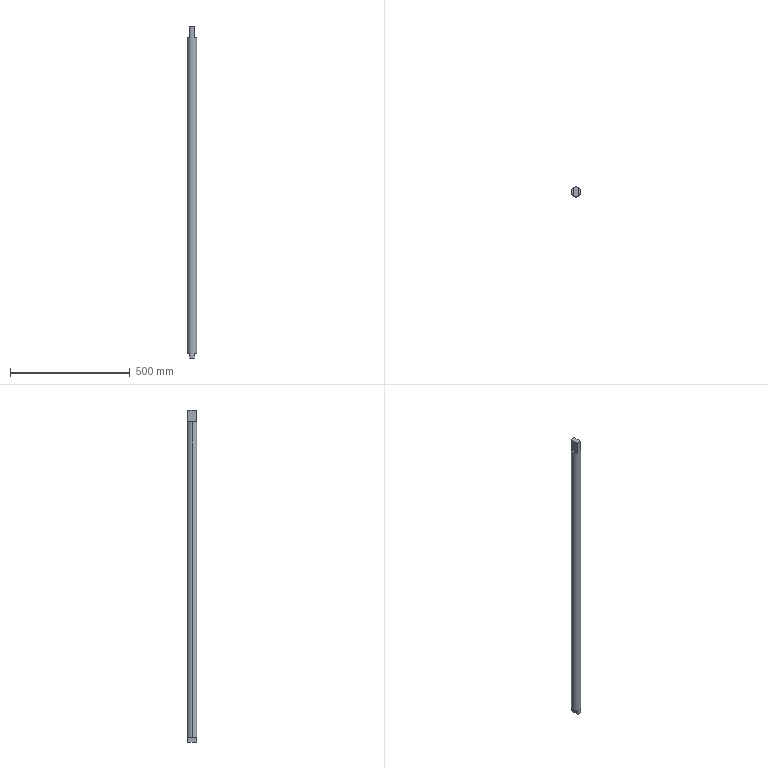Part | SolidWorks | 1 solid | 12 faces | box 40 x 40 x 1385 mm | volume 1706048 mm3 | plane 10 | cylinder 2 | commonest cylinder face diameters 40 x2
STEP:
#1=CARTESIAN_POINT('',(20.,0.,1280.));
#2=VERTEX_POINT('',#1);
#3=CARTESIAN_POINT('',(10.,17.321,1280.));
#4=VERTEX_POINT('',#3);
#5=CARTESIAN_POINT('',(0.,0.,1280.));
#6=DIRECTION('',(0.,0.,1.));
#7=DIRECTION('',(1.,0.,0.));
#8=AXIS2_PLACEMENT_3D('',#5,#6,#7);
#9=CIRCLE('',#8,20.);
#10=EDGE_CURVE('',#2,#4,#9,.T.);
#11=ORIENTED_EDGE('',*,*,#10,.F.);
#12=CARTESIAN_POINT('',(20.,0.,-35.));
#13=VERTEX_POINT('',#12);
#14=CARTESIAN_POINT('',(20.,0.,1280.));
#15=DIRECTION('',(0.,0.,-1.));
#16=VECTOR('',#15,1000.);
#17=LINE('',#14,#16);
#18=EDGE_CURVE('',#2,#13,#17,.T.);
#19=ORIENTED_EDGE('',*,*,#18,.T.);
#20=CARTESIAN_POINT('',(10.,17.321,-35.));
#21=VERTEX_POINT('',#20);
#22=CARTESIAN_POINT('',(0.,0.,-35.));
#23=DIRECTION('',(0.,0.,-1.));
#24=DIRECTION('',(-1.,0.,0.));
#25=AXIS2_PLACEMENT_3D('',#22,#23,#24);
#26=CIRCLE('',#25,20.);
#27=EDGE_CURVE('',#21,#13,#26,.T.);
#28=ORIENTED_EDGE('',*,*,#27,.F.);
#29=CARTESIAN_POINT('',(10.,17.321,-55.));
#30=VERTEX_POINT('',#29);
#31=CARTESIAN_POINT('',(10.,17.321,-55.));
#32=DIRECTION('',(0.,0.,1.));
#33=VECTOR('',#32,1000.);
#34=LINE('',#31,#33);
#35=EDGE_CURVE('',#30,#21,#34,.T.);
#36=ORIENTED_EDGE('',*,*,#35,.F.);
#37=CARTESIAN_POINT('',(-10.,17.321,-55.));
#38=VERTEX_POINT('',#37);
#39=CARTESIAN_POINT('',(0.,0.,-55.));
#40=DIRECTION('',(0.,0.,-1.));
#41=DIRECTION('',(-1.,0.,0.));
#42=AXIS2_PLACEMENT_3D('',#39,#40,#41);
#43=CIRCLE('',#42,20.);
#44=EDGE_CURVE('',#38,#30,#43,.T.);
#45=ORIENTED_EDGE('',*,*,#44,.F.);
#46=CARTESIAN_POINT('',(-10.,17.321,-35.));
#47=VERTEX_POINT('',#46);
#48=CARTESIAN_POINT('',(-10.,17.321,-55.));
#49=DIRECTION('',(0.,0.,1.));
#50=VECTOR('',#49,1000.);
#51=LINE('',#48,#50);
#52=EDGE_CURVE('',#38,#47,#51,.T.);
#53=ORIENTED_EDGE('',*,*,#52,.T.);
#54=CARTESIAN_POINT('',(-20.,0.,-35.));
#55=VERTEX_POINT('',#54);
#56=CARTESIAN_POINT('',(0.,0.,-35.));
#57=DIRECTION('',(0.,0.,-1.));
#58=DIRECTION('',(-1.,0.,0.));
#59=AXIS2_PLACEMENT_3D('',#56,#57,#58);
#60=CIRCLE('',#59,20.);
#61=EDGE_CURVE('',#55,#47,#60,.T.);
#62=ORIENTED_EDGE('',*,*,#61,.F.);
#63=CARTESIAN_POINT('',(-20.,0.,1280.));
#64=VERTEX_POINT('',#63);
#65=CARTESIAN_POINT('',(-20.,0.,1280.));
#66=DIRECTION('',(0.,0.,-1.));
#67=VECTOR('',#66,1000.);
#68=LINE('',#65,#67);
#69=EDGE_CURVE('',#64,#55,#68,.T.);
#70=ORIENTED_EDGE('',*,*,#69,.F.);
#71=CARTESIAN_POINT('',(-10.,17.321,1280.));
#72=VERTEX_POINT('',#71);
#73=CARTESIAN_POINT('',(0.,0.,1280.));
#74=DIRECTION('',(0.,0.,1.));
#75=DIRECTION('',(1.,0.,0.));
#76=AXIS2_PLACEMENT_3D('',#73,#74,#75);
#77=CIRCLE('',#76,20.);
#78=EDGE_CURVE('',#72,#64,#77,.T.);
#79=ORIENTED_EDGE('',*,*,#78,.F.);
#80=CARTESIAN_POINT('',(-10.,17.321,1330.));
#81=VERTEX_POINT('',#80);
#82=CARTESIAN_POINT('',(-10.,17.321,1330.));
#83=DIRECTION('',(0.,0.,-1.));
#84=VECTOR('',#83,1000.);
#85=LINE('',#82,#84);
#86=EDGE_CURVE('',#81,#72,#85,.T.);
#87=ORIENTED_EDGE('',*,*,#86,.F.);
#88=CARTESIAN_POINT('',(10.,17.321,1330.));
#89=VERTEX_POINT('',#88);
#90=CARTESIAN_POINT('',(0.,0.,1330.));
#91=DIRECTION('',(0.,0.,1.));
#92=DIRECTION('',(1.,0.,0.));
#93=AXIS2_PLACEMENT_3D('',#90,#91,#92);
#94=CIRCLE('',#93,20.);
#95=EDGE_CURVE('',#89,#81,#94,.T.);
#96=ORIENTED_EDGE('',*,*,#95,.F.);
#97=CARTESIAN_POINT('',(10.,17.321,1330.));
#98=DIRECTION('',(0.,0.,-1.));
#99=VECTOR('',#98,1000.);
#100=LINE('',#97,#99);
#101=EDGE_CURVE('',#89,#4,#100,.T.);
#102=ORIENTED_EDGE('',*,*,#101,.T.);
#103=EDGE_LOOP('',(#11,#19,#28,#36,#45,#53,#62,#70,#79,#87,#96,#102));
#104=FACE_OUTER_BOUND('',#103,.T.);
#105=CARTESIAN_POINT('',(0.,0.,1280.));
#106=DIRECTION('',(0.,0.,-1.));
#107=DIRECTION('',(-1.,0.,0.));
#108=AXIS2_PLACEMENT_3D('',#105,#106,#107);
#109=CYLINDRICAL_SURFACE('',#108,20.);
#110=ADVANCED_FACE('',(#104),#109,.T.);
#111=CARTESIAN_POINT('',(-10.,-17.321,-35.));
#112=VERTEX_POINT('',#111);
#113=CARTESIAN_POINT('',(0.,0.,-35.));
#114=DIRECTION('',(0.,0.,-1.));
#115=DIRECTION('',(-1.,0.,0.));
#116=AXIS2_PLACEMENT_3D('',#113,#114,#115);
#117=CIRCLE('',#116,20.);
#118=EDGE_CURVE('',#112,#55,#117,.T.);
#119=ORIENTED_EDGE('',*,*,#118,.T.);
#120=ORIENTED_EDGE('',*,*,#61,.T.);
#121=CARTESIAN_POINT('',(-10.,0.,-35.));
#122=DIRECTION('',(0.,-1.,0.));
#123=VECTOR('',#122,1000.);
#124=LINE('',#121,#123);
#125=EDGE_CURVE('',#47,#112,#124,.T.);
#126=ORIENTED_EDGE('',*,*,#125,.T.);
#127=EDGE_LOOP('',(#119,#120,#126));
#128=FACE_OUTER_BOUND('',#127,.T.);
#129=CARTESIAN_POINT('',(0.,0.,-35.));
#130=DIRECTION('',(0.,0.,-1.));
#131=DIRECTION('',(-1.,0.,0.));
#132=AXIS2_PLACEMENT_3D('',#129,#130,#131);
#133=PLANE('',#132);
#134=ADVANCED_FACE('',(#128),#133,.T.);
#135=CARTESIAN_POINT('',(10.,-17.321,-35.));
#136=VERTEX_POINT('',#135);
#137=CARTESIAN_POINT('',(10.,0.,-35.));
#138=DIRECTION('',(0.,-1.,0.));
#139=VECTOR('',#138,1000.);
#140=LINE('',#137,#139);
#141=EDGE_CURVE('',#21,#136,#140,.T.);
#142=ORIENTED_EDGE('',*,*,#141,.F.);
#143=ORIENTED_EDGE('',*,*,#27,.T.);
#144=CARTESIAN_POINT('',(0.,0.,-35.));
#145=DIRECTION('',(0.,0.,-1.));
#146=DIRECTION('',(-1.,0.,0.));
#147=AXIS2_PLACEMENT_3D('',#144,#145,#146);
#148=CIRCLE('',#147,20.);
#149=EDGE_CURVE('',#13,#136,#148,.T.);
#150=ORIENTED_EDGE('',*,*,#149,.T.);
#151=EDGE_LOOP('',(#142,#143,#150));
#152=FACE_OUTER_BOUND('',#151,.T.);
#153=CARTESIAN_POINT('',(0.,0.,-35.));
#154=DIRECTION('',(0.,0.,-1.));
#155=DIRECTION('',(-1.,0.,0.));
#156=AXIS2_PLACEMENT_3D('',#153,#154,#155);
#157=PLANE('',#156);
#158=ADVANCED_FACE('',(#152),#157,.T.);
#159=CARTESIAN_POINT('',(10.,-17.321,1280.));
#160=VERTEX_POINT('',#159);
#161=CARTESIAN_POINT('',(0.,0.,1280.));
#162=DIRECTION('',(0.,0.,1.));
#163=DIRECTION('',(1.,0.,0.));
#164=AXIS2_PLACEMENT_3D('',#161,#162,#163);
#165=CIRCLE('',#164,20.);
#166=EDGE_CURVE('',#160,#2,#165,.T.);
#167=ORIENTED_EDGE('',*,*,#166,.T.);
#168=ORIENTED_EDGE('',*,*,#10,.T.);
#169=CARTESIAN_POINT('',(10.,0.,1280.));
#170=DIRECTION('',(0.,-1.,0.));
#171=VECTOR('',#170,1000.);
#172=LINE('',#169,#171);
#173=EDGE_CURVE('',#4,#160,#172,.T.);
#174=ORIENTED_EDGE('',*,*,#173,.T.);
#175=EDGE_LOOP('',(#167,#168,#174));
#176=FACE_OUTER_BOUND('',#175,.T.);
#177=CARTESIAN_POINT('',(0.,0.,1280.));
#178=DIRECTION('',(0.,0.,1.));
#179=DIRECTION('',(1.,0.,0.));
#180=AXIS2_PLACEMENT_3D('',#177,#178,#179);
#181=PLANE('',#180);
#182=ADVANCED_FACE('',(#176),#181,.T.);
#183=ORIENTED_EDGE('',*,*,#18,.F.);
#184=ORIENTED_EDGE('',*,*,#166,.F.);
#185=CARTESIAN_POINT('',(10.,-17.321,1330.));
#186=VERTEX_POINT('',#185);
#187=CARTESIAN_POINT('',(10.,-17.321,1330.));
#188=DIRECTION('',(0.,0.,-1.));
#189=VECTOR('',#188,1000.);
#190=LINE('',#187,#189);
#191=EDGE_CURVE('',#186,#160,#190,.T.);
#192=ORIENTED_EDGE('',*,*,#191,.F.);
#193=CARTESIAN_POINT('',(-10.,-17.321,1330.));
#194=VERTEX_POINT('',#193);
#195=CARTESIAN_POINT('',(0.,0.,1330.));
#196=DIRECTION('',(0.,0.,1.));
#197=DIRECTION('',(1.,0.,0.));
#198=AXIS2_PLACEMENT_3D('',#195,#196,#197);
#199=CIRCLE('',#198,20.);
#200=EDGE_CURVE('',#194,#186,#199,.T.);
#201=ORIENTED_EDGE('',*,*,#200,.F.);
#202=CARTESIAN_POINT('',(-10.,-17.321,1280.));
#203=VERTEX_POINT('',#202);
#204=CARTESIAN_POINT('',(-10.,-17.321,1330.));
#205=DIRECTION('',(0.,0.,-1.));
#206=VECTOR('',#205,1000.);
#207=LINE('',#204,#206);
#208=EDGE_CURVE('',#194,#203,#207,.T.);
#209=ORIENTED_EDGE('',*,*,#208,.T.);
#210=CARTESIAN_POINT('',(0.,0.,1280.));
#211=DIRECTION('',(0.,0.,1.));
#212=DIRECTION('',(1.,0.,0.));
#213=AXIS2_PLACEMENT_3D('',#210,#211,#212);
#214=CIRCLE('',#213,20.);
#215=EDGE_CURVE('',#64,#203,#214,.T.);
#216=ORIENTED_EDGE('',*,*,#215,.F.);
#217=ORIENTED_EDGE('',*,*,#69,.T.);
#218=ORIENTED_EDGE('',*,*,#118,.F.);
#219=CARTESIAN_POINT('',(-10.,-17.321,-55.));
#220=VERTEX_POINT('',#219);
#221=CARTESIAN_POINT('',(-10.,-17.321,-55.));
#222=DIRECTION('',(0.,0.,1.));
#223=VECTOR('',#222,1000.);
#224=LINE('',#221,#223);
#225=EDGE_CURVE('',#220,#112,#224,.T.);
#226=ORIENTED_EDGE('',*,*,#225,.F.);
#227=CARTESIAN_POINT('',(10.,-17.321,-55.));
#228=VERTEX_POINT('',#227);
#229=CARTESIAN_POINT('',(0.,0.,-55.));
#230=DIRECTION('',(0.,0.,-1.));
#231=DIRECTION('',(-1.,0.,0.));
#232=AXIS2_PLACEMENT_3D('',#229,#230,#231);
#233=CIRCLE('',#232,20.);
#234=EDGE_CURVE('',#228,#220,#233,.T.);
#235=ORIENTED_EDGE('',*,*,#234,.F.);
#236=CARTESIAN_POINT('',(10.,-17.321,-55.));
#237=DIRECTION('',(0.,0.,1.));
#238=VECTOR('',#237,1000.);
#239=LINE('',#236,#238);
#240=EDGE_CURVE('',#228,#136,#239,.T.);
#241=ORIENTED_EDGE('',*,*,#240,.T.);
#242=ORIENTED_EDGE('',*,*,#149,.F.);
#243=EDGE_LOOP('',(#183,#184,#192,#201,#209,#216,#217,#218,#226,#235,#241,#242));
#244=FACE_OUTER_BOUND('',#243,.T.);
#245=CARTESIAN_POINT('',(0.,0.,1280.));
#246=DIRECTION('',(0.,0.,-1.));
#247=DIRECTION('',(-1.,0.,0.));
#248=AXIS2_PLACEMENT_3D('',#245,#246,#247);
#249=CYLINDRICAL_SURFACE('',#248,20.);
#250=ADVANCED_FACE('',(#244),#249,.T.);
#251=CARTESIAN_POINT('',(-10.,0.,1280.));
#252=DIRECTION('',(0.,-1.,0.));
#253=VECTOR('',#252,1000.);
#254=LINE('',#251,#253);
#255=EDGE_CURVE('',#72,#203,#254,.T.);
#256=ORIENTED_EDGE('',*,*,#255,.F.);
#257=ORIENTED_EDGE('',*,*,#78,.T.);
#258=ORIENTED_EDGE('',*,*,#215,.T.);
#259=EDGE_LOOP('',(#256,#257,#258));
#260=FACE_OUTER_BOUND('',#259,.T.);
#261=CARTESIAN_POINT('',(0.,0.,1280.));
#262=DIRECTION('',(0.,0.,1.));
#263=DIRECTION('',(1.,0.,0.));
#264=AXIS2_PLACEMENT_3D('',#261,#262,#263);
#265=PLANE('',#264);
#266=ADVANCED_FACE('',(#260),#265,.T.);
#267=ORIENTED_EDGE('',*,*,#173,.F.);
#268=ORIENTED_EDGE('',*,*,#101,.F.);
#269=CARTESIAN_POINT('',(10.,0.,1330.));
#270=DIRECTION('',(0.,-1.,0.));
#271=VECTOR('',#270,1000.);
#272=LINE('',#269,#271);
#273=EDGE_CURVE('',#89,#186,#272,.T.);
#274=ORIENTED_EDGE('',*,*,#273,.T.);
#275=ORIENTED_EDGE('',*,*,#191,.T.);
#276=EDGE_LOOP('',(#267,#268,#274,#275));
#277=FACE_OUTER_BOUND('',#276,.T.);
#278=CARTESIAN_POINT('',(10.,0.,1330.));
#279=DIRECTION('',(1.,0.,0.));
#280=DIRECTION('',(0.,0.,-1.));
#281=AXIS2_PLACEMENT_3D('',#278,#279,#280);
#282=PLANE('',#281);
#283=ADVANCED_FACE('',(#277),#282,.T.);
#284=ORIENTED_EDGE('',*,*,#255,.T.);
#285=ORIENTED_EDGE('',*,*,#208,.F.);
#286=CARTESIAN_POINT('',(-10.,0.,1330.));
#287=DIRECTION('',(0.,-1.,0.));
#288=VECTOR('',#287,1000.);
#289=LINE('',#286,#288);
#290=EDGE_CURVE('',#81,#194,#289,.T.);
#291=ORIENTED_EDGE('',*,*,#290,.F.);
#292=ORIENTED_EDGE('',*,*,#86,.T.);
#293=EDGE_LOOP('',(#284,#285,#291,#292));
#294=FACE_OUTER_BOUND('',#293,.T.);
#295=CARTESIAN_POINT('',(-10.,0.,1330.));
#296=DIRECTION('',(1.,0.,0.));
#297=DIRECTION('',(0.,0.,-1.));
#298=AXIS2_PLACEMENT_3D('',#295,#296,#297);
#299=PLANE('',#298);
#300=ADVANCED_FACE('',(#294),#299,.F.);
#301=ORIENTED_EDGE('',*,*,#273,.F.);
#302=ORIENTED_EDGE('',*,*,#95,.T.);
#303=ORIENTED_EDGE('',*,*,#290,.T.);
#304=ORIENTED_EDGE('',*,*,#200,.T.);
#305=EDGE_LOOP('',(#301,#302,#303,#304));
#306=FACE_OUTER_BOUND('',#305,.T.);
#307=CARTESIAN_POINT('',(0.,0.,1330.));
#308=DIRECTION('',(0.,0.,1.));
#309=DIRECTION('',(1.,0.,0.));
#310=AXIS2_PLACEMENT_3D('',#307,#308,#309);
#311=PLANE('',#310);
#312=ADVANCED_FACE('',(#306),#311,.T.);
#313=ORIENTED_EDGE('',*,*,#141,.T.);
#314=ORIENTED_EDGE('',*,*,#240,.F.);
#315=CARTESIAN_POINT('',(10.,0.,-55.));
#316=DIRECTION('',(0.,-1.,0.));
#317=VECTOR('',#316,1000.);
#318=LINE('',#315,#317);
#319=EDGE_CURVE('',#30,#228,#318,.T.);
#320=ORIENTED_EDGE('',*,*,#319,.F.);
#321=ORIENTED_EDGE('',*,*,#35,.T.);
#322=EDGE_LOOP('',(#313,#314,#320,#321));
#323=FACE_OUTER_BOUND('',#322,.T.);
#324=CARTESIAN_POINT('',(10.,0.,-55.));
#325=DIRECTION('',(-1.,0.,0.));
#326=DIRECTION('',(0.,0.,1.));
#327=AXIS2_PLACEMENT_3D('',#324,#325,#326);
#328=PLANE('',#327);
#329=ADVANCED_FACE('',(#323),#328,.F.);
#330=ORIENTED_EDGE('',*,*,#125,.F.);
#331=ORIENTED_EDGE('',*,*,#52,.F.);
#332=CARTESIAN_POINT('',(-10.,0.,-55.));
#333=DIRECTION('',(0.,-1.,0.));
#334=VECTOR('',#333,1000.);
#335=LINE('',#332,#334);
#336=EDGE_CURVE('',#38,#220,#335,.T.);
#337=ORIENTED_EDGE('',*,*,#336,.T.);
#338=ORIENTED_EDGE('',*,*,#225,.T.);
#339=EDGE_LOOP('',(#330,#331,#337,#338));
#340=FACE_OUTER_BOUND('',#339,.T.);
#341=CARTESIAN_POINT('',(-10.,0.,-55.));
#342=DIRECTION('',(-1.,0.,0.));
#343=DIRECTION('',(0.,0.,1.));
#344=AXIS2_PLACEMENT_3D('',#341,#342,#343);
#345=PLANE('',#344);
#346=ADVANCED_FACE('',(#340),#345,.T.);
#347=ORIENTED_EDGE('',*,*,#44,.T.);
#348=ORIENTED_EDGE('',*,*,#319,.T.);
#349=ORIENTED_EDGE('',*,*,#234,.T.);
#350=ORIENTED_EDGE('',*,*,#336,.F.);
#351=EDGE_LOOP('',(#347,#348,#349,#350));
#352=FACE_OUTER_BOUND('',#351,.T.);
#353=CARTESIAN_POINT('',(0.,0.,-55.));
#354=DIRECTION('',(0.,0.,-1.));
#355=DIRECTION('',(-1.,0.,0.));
#356=AXIS2_PLACEMENT_3D('',#353,#354,#355);
#357=PLANE('',#356);
#358=ADVANCED_FACE('',(#352),#357,.T.);
#359=CLOSED_SHELL('',(#110,#134,#158,#182,#250,#266,#283,#300,#312,#329,#346,#358));
#360=MANIFOLD_SOLID_BREP('',#359);
#361=CARTESIAN_POINT('',(0.,0.,0.));
#362=DIRECTION('',(0.,0.,1.));
#363=DIRECTION('',(1.,0.,0.));
#364=AXIS2_PLACEMENT_3D('',#361,#362,#363);
#365=(LENGTH_UNIT()NAMED_UNIT(*)SI_UNIT(.MILLI.,.METRE.));
#366=UNCERTAINTY_MEASURE_WITH_UNIT(LENGTH_MEASURE(0.00001),#365,'','');
#367=(NAMED_UNIT(*)PLANE_ANGLE_UNIT()SI_UNIT($,.RADIAN.));
#368=(NAMED_UNIT(*)SI_UNIT($,.STERADIAN.)SOLID_ANGLE_UNIT());
#369=(GEOMETRIC_REPRESENTATION_CONTEXT(3)GLOBAL_UNCERTAINTY_ASSIGNED_CONTEXT((#366))GLOBAL_UNIT_ASSIGNED_CONTEXT((#365,#367,#368))REPRESENTATION_CONTEXT('',''));
#370=ADVANCED_BREP_SHAPE_REPRESENTATION('',(#360,#364),#369);